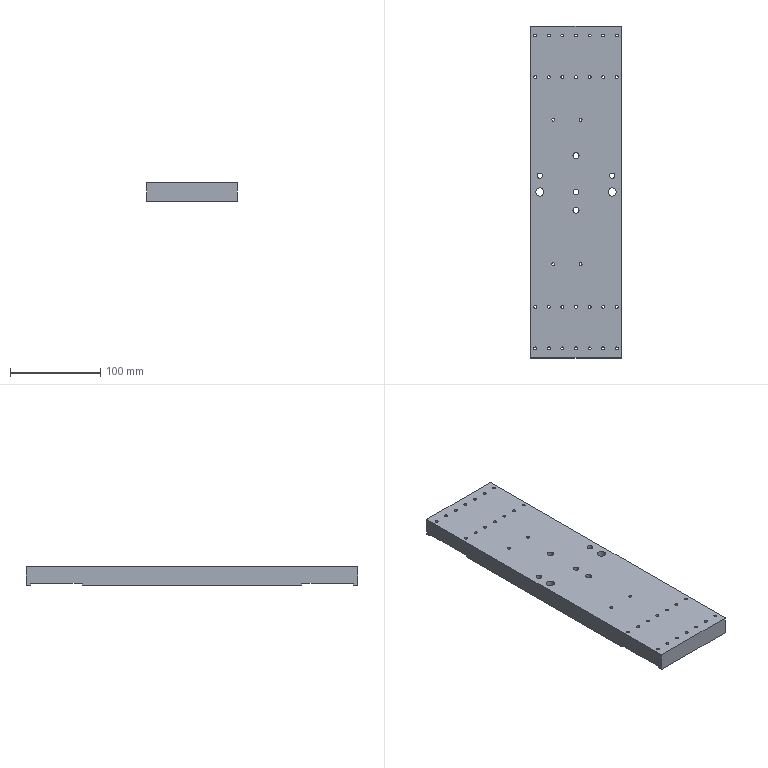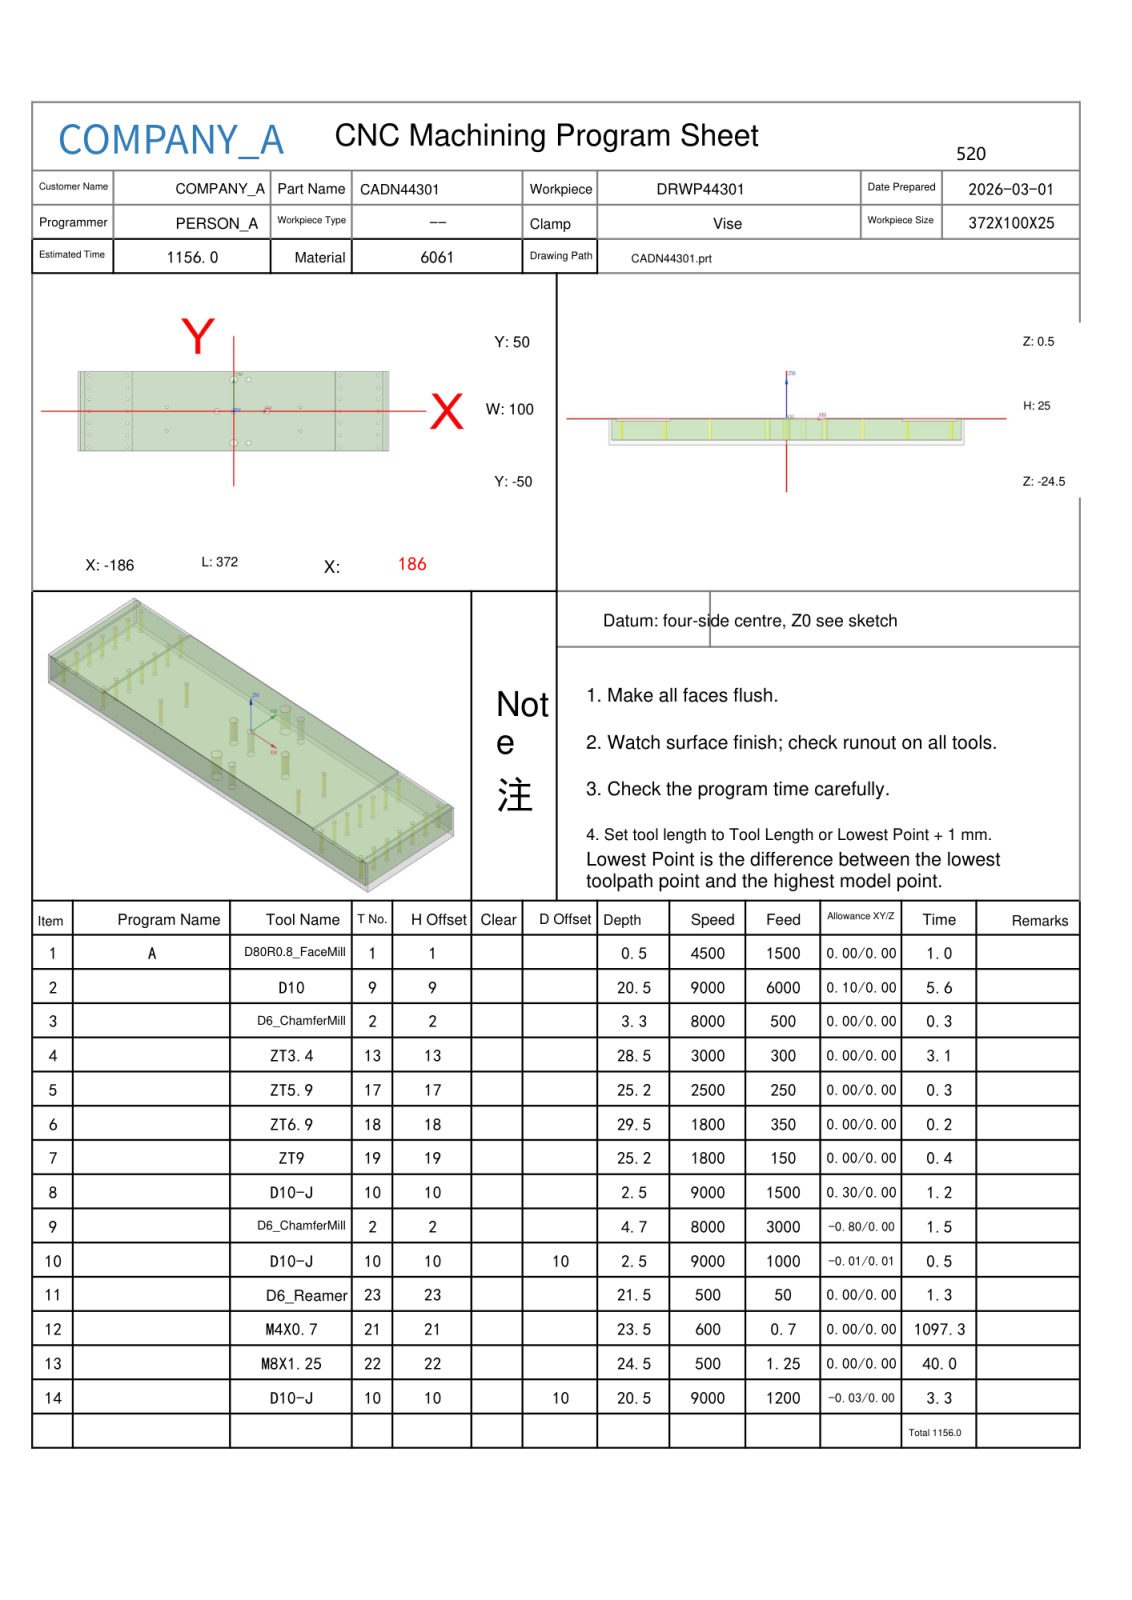NC program | NX | posted by the shop | part box 100 x 367 x 20 mm
Whole program:
%
O0001
(Machine time: 2248.24 MIN)
(===Total Tool:11===)
(T1=D80R0.8 FaceMill D=80.  R=0.8  D-  H01 Z=0.    )
(T9=D10     D=10.  R=0.   D-  H09 Z=-20.  )
(T2=D6_ChamferMill   D=6.   R=0.   D-  H02 Z=-4.2  )
(T13=ZT3.4  D=3.4  DR_a=118 D-  H13 Z=-28.  )
(T17=ZT5.9  D=5.9  DR_a=120 D-  H17 Z=-24.7 )
(T18=ZT6.9  D=6.9  DR_a=120 D-  H18 Z=-29.  )
(T19=ZT9    D=9.   DR_a=118 D-  H19 Z=-24.7 )
(T10=D10-J  D=10.  R=0.   D-  H10 Z=-20.  )
(T23=D6_Reamer   D=6.   DR_a=180 D23 H23 Z=-21.  )
(T21=M4X0.7 D=3.3  DR_a=180 D-  H21 Z=-23.  )
(T22=M8X1.25 D=6.8  DR_a=180 D-  H22 Z=-24.  )
G80 G90 G17 G49 G40
G91 G28 Z0
M01
N1 T01 M06
(D80R0.8 FaceMill  D=80. R=0.8 H=01 ce=0.00 di=0.00)
G00 G90 G54 X-228.5 Y45. M03 S4500
G43 H01 Z50.
M08
Z2.
G01 Z0.0 F1500.
X-223.5
X223.5
Y0.0
X-223.5
Y-45.
X223.5
X228.5
Z2.
G00 Z50.
G91 G28 Z0.0
M05
M09
G91 G28 Z0.0
M01
N2 T09 M06
(D10  D=10. R=0. H=09 ce=0.10 di=0.00)
G00 G90 G54 X0.0 Y55.1 M03 S8000
G43 H09 Z50.
M08
Z.5
G01 X183.5 Z.35 F6000.
G02 X188.6 Y50. Z.344 I0.0 J-5.1
G01 Y-50. Z.262
G02 X183.5 Y-55.1 Z.256 I-5.1 J0.0
G01 X-183.5 Z-.044
G02 X-188.6 Y-50. Z-.051 I0.0 J5.1
G01 Y50. Z-.132
G02 X-183.5 Y55.1 Z-.139 I5.1 J0.0
G01 X183.5 Z-.438
G02 X188.6 Y50. Z-.445 I0.0 J-5.1
G01 Y-50. Z-.526
G02 X183.5 Y-55.1 Z-.533 I-5.1 J0.0
G01 X-183.5 Z-.832
G02 X-188.6 Y-50. Z-.839 I0.0 J5.1
G01 Y50. Z-.921
G02 X-183.5 Y55.1 Z-.927 I5.1 J0.0
G01 X183.5 Z-1.227
G02 X188.6 Y50. Z-1.233 I0.0 J-5.1
G01 Y-50. Z-1.315
G02 X183.5 Y-55.1 Z-1.321 I-5.1 J0.0
G01 X-183.5 Z-1.621
G02 X-188.6 Y-50. Z-1.627 I0.0 J5.1
G01 Y50. Z-1.709
G02 X-183.5 Y55.1 Z-1.716 I5.1 J0.0
G01 X183.5 Z-2.015
G02 X188.6 Y50. Z-2.022 I0.0 J-5.1
G01 Y-50. Z-2.103
G02 X183.5 Y-55.1 Z-2.11 I-5.1 J0.0
G01 X-183.5 Z-2.409
G02 X-188.6 Y-50. Z-2.416 I0.0 J5.1
G01 Y50. Z-2.498
G02 X-183.5 Y55.1 Z-2.504 I5.1 J0.0
G01 X183.5 Z-2.804
G02 X188.6 Y50. Z-2.81 I0.0 J-5.1
G01 Y-50. Z-2.892
G02 X183.5 Y-55.1 Z-2.898 I-5.1 J0.0
G01 X-183.5 Z-3.198
G02 X-188.6 Y-50. Z-3.204 I0.0 J5.1
G01 Y50. Z-3.286
G02 X-183.5 Y55.1 Z-3.293 I5.1 J0.0
G01 X183.5 Z-3.592
G02 X188.6 Y50. Z-3.599 I0.0 J-5.1
G01 Y-50. Z-3.68
G02 X183.5 Y-55.1 Z-3.687 I-5.1 J0.0
G01 X-183.5 Z-3.986
G02 X-188.6 Y-50. Z-3.993 I0.0 J5.1
G01 Y50. Z-4.074
G02 X-183.5 Y55.1 Z-4.081 I5.1 J0.0
G01 X183.5 Z-4.381
G02 X188.6 Y50. Z-4.387 I0.0 J-5.1
G01 Y-50. Z-4.469
G02 X183.5 Y-55.1 Z-4.475 I-5.1 J0.0
G01 X-183.5 Z-4.775
G02 X-188.6 Y-50. Z-4.781 I0.0 J5.1
G01 Y50. Z-4.863
G02 X-183.5 Y55.1 Z-4.869 I5.1 J0.0
G01 X183.5 Z-5.169
G02 X188.6 Y50. Z-5.176 I0.0 J-5.1
G01 Y-50. Z-5.257
G02 X183.5 Y-55.1 Z-5.264 I-5.1 J0.0
G01 X-183.5 Z-5.563
G02 X-188.6 Y-50. Z-5.57 I0.0 J5.1
G01 Y50. Z-5.651
G02 X-183.5 Y55.1 Z-5.658 I5.1 J0.0
G01 X183.5 Z-5.957
G02 X188.6 Y50. Z-5.964 I0.0 J-5.1
G01 Y-50. Z-6.046
G02 X183.5 Y-55.1 Z-6.052 I-5.1 J0.0
G01 X-183.5 Z-6.352
G02 X-188.6 Y-50. Z-6.358 I0.0 J5.1
G01 Y50. Z-6.44
G02 X-183.5 Y55.1 Z-6.446 I5.1 J0.0
G01 X183.5 Z-6.746
G02 X188.6 Y50. Z-6.752 I0.0 J-5.1
G01 Y-50. Z-6.834
G02 X183.5 Y-55.1 Z-6.841 I-5.1 J0.0
G01 X-183.5 Z-7.14
G02 X-188.6 Y-50. Z-7.147 I0.0 J5.1
G01 Y50. Z-7.228
G02 X-183.5 Y55.1 Z-7.235 I5.1 J0.0
G01 X183.5 Z-7.534
G02 X188.6 Y50. Z-7.541 I0.0 J-5.1
G01 Y-50. Z-7.623
G02 X183.5 Y-55.1 Z-7.629 I-5.1 J0.0
G01 X-183.5 Z-7.929
G02 X-188.6 Y-50. Z-7.935 I0.0 J5.1
G01 Y50. Z-8.017
G02 X-183.5 Y55.1 Z-8.023 I5.1 J0.0
G01 X183.5 Z-8.323
G02 X188.6 Y50. Z-8.329 I0.0 J-5.1
G01 Y-50. Z-8.411
G02 X183.5 Y-55.1 Z-8.418 I-5.1 J0.0
G01 X-183.5 Z-8.717
G02 X-188.6 Y-50. Z-8.724 I0.0 J5.1
G01 Y50. Z-8.805
G02 X-183.5 Y55.1 Z-8.812 I5.1 J0.0
G01 X183.5 Z-9.111
G02 X188.6 Y50. Z-9.118 I0.0 J-5.1
G01 Y-50. Z-9.199
G02 X183.5 Y-55.1 Z-9.206 I-5.1 J0.0
G01 X-183.5 Z-9.506
G02 X-188.6 Y-50. Z-9.512 I0.0 J5.1
G01 Y50. Z-9.594
G02 X-183.5 Y55.1 Z-9.6 I5.1 J0.0
G01 X183.5 Z-9.9
G02 X188.6 Y50. Z-9.906 I0.0 J-5.1
G01 Y-50. Z-9.988
G02 X183.5 Y-55.1 Z-9.994 I-5.1 J0.0
G01 X-183.5 Z-10.294
G02 X-188.6 Y-50. Z-10.301 I0.0 J5.1
G01 Y50. Z-10.382
G02 X-183.5 Y55.1 Z-10.389 I5.1 J0.0
G01 X183.5 Z-10.688
G02 X188.6 Y50. Z-10.695 I0.0 J-5.1
G01 Y-50. Z-10.776
G02 X183.5 Y-55.1 Z-10.783 I-5.1 J0.0
G01 X-183.5 Z-11.082
G02 X-188.6 Y-50. Z-11.089 I0.0 J5.1
G01 Y50. Z-11.171
G02 X-183.5 Y55.1 Z-11.177 I5.1 J0.0
G01 X183.5 Z-11.477
G02 X188.6 Y50. Z-11.483 I0.0 J-5.1
G01 Y-50. Z-11.565
G02 X183.5 Y-55.1 Z-11.571 I-5.1 J0.0
G01 X-183.5 Z-11.871
G02 X-188.6 Y-50. Z-11.877 I0.0 J5.1
G01 Y50. Z-11.959
G02 X-183.5 Y55.1 Z-11.966 I5.1 J0.0
G01 X183.5 Z-12.265
G02 X188.6 Y50. Z-12.272 I0.0 J-5.1
G01 Y-50. Z-12.353
G02 X183.5 Y-55.1 Z-12.36 I-5.1 J0.0
G01 X-183.5 Z-12.659
G02 X-188.6 Y-50. Z-12.666 I0.0 J5.1
G01 Y50. Z-12.748
G02 X-183.5 Y55.1 Z-12.754 I5.1 J0.0
G01 X183.5 Z-13.054
G02 X188.6 Y50. Z-13.06 I0.0 J-5.1
G01 Y-50. Z-13.142
G02 X183.5 Y-55.1 Z-13.148 I-5.1 J0.0
G01 X-183.5 Z-13.448
G02 X-188.6 Y-50. Z-13.454 I0.0 J5.1
G01 Y50. Z-13.536
G02 X-183.5 Y55.1 Z-13.543 I5.1 J0.0
G01 X183.5 Z-13.842
G02 X188.6 Y50. Z-13.849 I0.0 J-5.1
G01 Y-50. Z-13.93
G02 X183.5 Y-55.1 Z-13.937 I-5.1 J0.0
G01 X-183.5 Z-14.236
G02 X-188.6 Y-50. Z-14.243 I0.0 J5.1
G01 Y50. Z-14.324
G02 X-183.5 Y55.1 Z-14.331 I5.1 J0.0
G01 X183.5 Z-14.631
G02 X188.6 Y50. Z-14.637 I0.0 J-5.1
G01 Y-50. Z-14.719
G02 X183.5 Y-55.1 Z-14.725 I-5.1 J0.0
G01 X-183.5 Z-15.025
G02 X-188.6 Y-50. Z-15.031 I0.0 J5.1
G01 Y50. Z-15.113
G02 X-183.5 Y55.1 Z-15.119 I5.1 J0.0
G01 X183.5 Z-15.419
G02 X188.6 Y50. Z-15.426 I0.0 J-5.1
G01 Y-50. Z-15.507
G02 X183.5 Y-55.1 Z-15.514 I-5.1 J0.0
G01 X-183.5 Z-15.813
G02 X-188.6 Y-50. Z-15.82 I0.0 J5.1
G01 Y50. Z-15.901
G02 X-183.5 Y55.1 Z-15.908 I5.1 J0.0
G01 X183.5 Z-16.207
G02 X188.6 Y50. Z-16.214 I0.0 J-5.1
G01 Y-50. Z-16.296
G02 X183.5 Y-55.1 Z-16.302 I-5.1 J0.0
G01 X-183.5 Z-16.602
G02 X-188.6 Y-50. Z-16.608 I0.0 J5.1
G01 Y50. Z-16.69
G02 X-183.5 Y55.1 Z-16.696 I5.1 J0.0
G01 X183.5 Z-16.996
G02 X188.6 Y50. Z-17.002 I0.0 J-5.1
G01 Y-50. Z-17.084
G02 X183.5 Y-55.1 Z-17.091 I-5.1 J0.0
G01 X-183.5 Z-17.39
G02 X-188.6 Y-50. Z-17.397 I0.0 J5.1
G01 Y50. Z-17.478
G02 X-183.5 Y55.1 Z-17.485 I5.1 J0.0
G01 X183.5 Z-17.784
G02 X188.6 Y50. Z-17.791 I0.0 J-5.1
G01 Y-50. Z-17.873
G02 X183.5 Y-55.1 Z-17.879 I-5.1 J0.0
G01 X-183.5 Z-18.179
G02 X-188.6 Y-50. Z-18.185 I0.0 J5.1
G01 Y50. Z-18.267
G02 X-183.5 Y55.1 Z-18.273 I5.1 J0.0
G01 X183.5 Z-18.573
G02 X188.6 Y50. Z-18.579 I0.0 J-5.1
G01 Y-50. Z-18.661
G02 X183.5 Y-55.1 Z-18.668 I-5.1 J0.0
G01 X-183.5 Z-18.967
G02 X-188.6 Y-50. Z-18.974 I0.0 J5.1
G01 Y50. Z-19.055
G02 X-183.5 Y55.1 Z-19.062 I5.1 J0.0
G01 X183.5 Z-19.361
G02 X188.6 Y50. Z-19.368 I0.0 J-5.1
G01 Y-50. Z-19.449
G02 X183.5 Y-55.1 Z-19.456 I-5.1 J0.0
G01 X-183.5 Z-19.756
G02 X-188.6 Y-50. Z-19.762 I0.0 J5.1
G01 Y50. Z-19.844
G02 X-183.5 Y55.1 Z-19.85 I5.1 J0.0
G01 X0.0 Z-20.
X183.5
G02 X188.6 Y50. I0.0 J-5.1
G01 Y-50.
G02 X183.5 Y-55.1 I-5.1 J0.0
G01 X-183.5
G02 X-188.6 Y-50. I0.0 J5.1
G01 Y50.
G02 X-183.5 Y55.1 I5.1 J0.0
G01 X0.0
X.5
Z-19.
G00 Z50.
G00 G90 X-150. Y58. M03 S9000
Z50.
Z.025
G01 Z-.475 F6000.
Y51.
X-126.6
Y-51.
X-173.4
Y51.
X-150.
Y44.
X-133.6
Y-44.
X-166.4
Y44.
X-150.
Y37.
X-140.6
Y-37.
X-159.4
Y37.
X-150.
Y30.
X-147.6
Y-30.
X-152.4
Y30.
X-150.
X-149.5
Z.025
G00 Z.5
X-150. Y58.
Z-.45
G01 Z-.95
Y51.
X-126.6
Y-51.
X-173.4
Y51.
X-150.
Y44.
X-133.6
Y-44.
X-166.4
Y44.
X-150.
Y37.
X-140.6
Y-37.
X-159.4
Y37.
X-150.
Y30.
X-147.6
Y-30.
X-152.4
Y30.
X-150.
X-149.5
Z-.45
G00 Z.025
X-150. Y58.
Z-.925
G01 Z-1.425
Y51.
X-126.6
Y-51.
X-173.4
Y51.
X-150.
Y44.
X-133.6
Y-44.
X-166.4
Y44.
X-150.
Y37.
X-140.6
Y-37.
X-159.4
Y37.
X-150.
Y30.
X-147.6
Y-30.
X-152.4
Y30.
X-150.
X-149.5
Z-.925
G00 Z-.45
X-150. Y58.
Z-1.4
G01 Z-1.9
Y51.
X-126.6
Y-51.
X-173.4
Y51.
X-150.
Y44.
X-133.6
Y-44.
X-166.4
Y44.
X-150.
Y37.
X-140.6
Y-37.
X-159.4
Y37.
X-150.
Y30.
X-147.6
Y-30.
X-152.4
Y30.
X-150.
X-149.5
Z-1.4
G00 Z50.
X150. Y58.
Z.025
G01 Z-.475
Y51.
X173.4
Y-51.
X126.6
Y51.
X150.
Y44.
X166.4
Y-44.
X133.6
Y44.
X150.
Y37.
X159.4
Y-37.
X140.6
Y37.
X150.
Y30.
X152.4
Y-30.
X147.6
Y30.
X150.
X150.5
Z.025
G00 Z.5
X150. Y58.
Z-.45
G01 Z-.95
Y51.
X173.4
Y-51.
X126.6
Y51.
X150.
Y44.
X166.4
Y-44.
X133.6
Y44.
X150.
Y37.
X159.4
Y-37.
X140.6
Y37.
X150.
Y30.
X152.4
Y-30.
X147.6
Y30.
X150.
X150.5
Z-.45
G00 Z.025
X150. Y58.
Z-.925
G01 Z-1.425
Y51.
X173.4
Y-51.
X126.6
Y51.
X150.
Y44.
X166.4
Y-44.
X133.6
Y44.
X150.
Y37.
X159.4
Y-37.
X140.6
Y37.
X150.
Y30.
X152.4
Y-30.
X147.6
Y30.
X150.
X150.5
Z-.925
G00 Z-.45
X150. Y58.
Z-1.4
G01 Z-1.9
Y51.
X173.4
Y-51.
X126.6
Y51.
X150.
Y44.
X166.4
Y-44.
X133.6
Y44.
X150.
Y37.
X159.4
Y-37.
X140.6
Y37.
X150.
Y30.
X152.4
Y-30.
X147.6
Y30.
X150.
X150.5
Z-1.4
G00 Z50.
G91 G28 Z0.0
M05
M09
G91 G28 Z0.0
M01
N3 T02 M06
(D6_ChamferMill  D=6. R=0. H=02 ce=0.00 di=0.10)
G00 G90 G54 X173. Y-45. M03 S8000
G43 H02 Z50.
M08
G98 G81 X173. Y-45. Z-2.8 R-1. F500.
Y-30.
Y-15.
Y0.0
Y15.
Y30.
Y45.
X127.
Y30.
Y15.
Y0.0
Y-15.
Y-30.
Y-45.
X80. Y-25. Z-.8 R1.
Y5.
X40. Y0.0
X18. Y40.
X0.0
Y0.0
X18. Y-40.
X0.0
X-20. Y0.0
X-80. Y-25.
Y5.
X-127. Y45. Z-2.8 R-1.
Y30.
Y15.
Y0.0
Y-15.
Y-30.
Y-45.
X-173.
Y-30.
Y-15.
Y0.0
Y15.
Y30.
Y45.
G80
G00 Z50.
G91 G28 Z0.0
M05
M09
G91 G28 Z0.0
M01
N4 T13 M06
(ZT3.4 D=3.4 DR_a=118 H=13)
G00 G90 G54 X-173. Y-45. M03 S3000
G43 H13 Z50.
M08
G98 G83 X-173. Y-45. Z-28. R-1. F300. Q2.
Y-30.
Y-15.
Y0.0
Y15.
Y30.
Y45.
X-127.
Y30.
Y15.
Y0.0
Y-15.
Y-30.
Y-45.
X-80. Y-25. Z-26. R1.
Y5.
X80.
Y-25.
X127. Y-45. Z-28. R-1.
Y-30.
Y-15.
Y0.0
Y15.
Y30.
Y45.
X173.
Y30.
Y15.
Y0.0
Y-15.
Y-30.
Y-45.
G80
G00 Z50.
G91 G28 Z0.0
M05
M09
G91 G28 Z0.0
M01
N5 T17 M06
(ZT5.9 D=5.9 DR_a=120 H=17)
G00 G90 G54 X18. Y40. M03 S2500
G43 H17 Z50.
M08
G98 G83 X18. Y40. Z-24.703 R1. F250. Q2.
X0.0 Y0.0
X18. Y-40.
G80
G00 Z50.
G91 G28 Z0.0
M05
M09
G91 G28 Z0.0
M01
N6 T18 M06
(ZT6.9 D=6.9 DR_a=120 H=18)
G00 G90 G54 X-20. Y0.0 M03 S1800
G43 H18 Z50.
M08
G98 G83 X-20. Y0.0 Z-29. R1. F350. Q3.
X40.
G80
G00 Z50.
G91 G28 Z0.0
M05
M09
G91 G28 Z0.0
M01
N7 T19 M06
(ZT9 D=9. DR_a=118 H=19)
G00 G90 G54 X0.0 Y40. M03 S1800
G43 H19 Z50.
M08
G98 G83 X0.0 Y40. Z-24.704 R1. F150. Q3.
Y-40.
G80
G00 Z50.
G91 G28 Z0.0
M05
M09
G91 G28 Z0.0
M01
N8 T10 M06
(D10-J  D=10. R=0. H=10 ce=0.30 di=0.00)
G00 G90 G54 X-150. Y58. M03 S9000
G43 H10 Z50.
M08
Z-1.5
G01 Z-2. F1500.
Y51.
X-126.8
Y-51.
X-173.2
Y51.
X-150.
Y44.
X-133.8
Y-44.
X-166.2
Y44.
X-150.
Y37.
X-140.8
Y-37.
X-159.2
Y37.
X-150.
Y30.
X-147.8
Y-30.
X-152.2
Y30.
X-150.
X-149.5
Y36.
Z-1.5
G00 Z50.
X150. Y58.
Z-1.5
G01 Z-2.
Y51.
X173.2
Y-51.
X126.8
Y51.
X150.
Y44.
X166.2
Y-44.
X133.8
Y44.
X150.
Y37.
X159.2
Y-37.
X140.8
Y37.
X150.
Y30.
X152.2
Y-30.
X147.8
Y30.
X150.
X150.5
Y36.
Z-1.5
G00 Z50.
G91 G28 Z0.0
M05
M09
G91 G28 Z0.0
M01
N9 T02 M06
(D6_ChamferMill  D=6. R=0. H=02 ce=0.00 di=0.00)
G00 G90 G54 X176.372 Y-.25 M03 S8000
G43 H02 Z50.
M08
Z2.099
G01 Z-1.5 F3000.
G03 X176.672 Y-.33 I.3 J.52
X177.192 Y-.03 I0.0 J.6
G01 X177.2 Y0.0
Y50.
G02 X178.5 Y51.3 I1.3 J0.0
G01 X183.5
G02 X184.8 Y50. I0.0 J-1.3
G01 Y-50.
G02 X183.5 Y-51.3 I-1.3 J0.0
G01 X178.5
G02 X177.2 Y-50. I0.0 J1.3
G01 Y0.0
X177.192 Y.03
G03 X176.672 Y.33 I-.52 J-.3
X176.372 Y.25 I0.0 J-.6
G01 Z2.099
G00 Z50.
X.25 Y-52.128
Z2.099
G01 Z-1.5
G03 X.33 Y-51.828 I-.52 J.3
X.03 Y-51.308 I-.6 J0.0
G01 X0.0 Y-51.3
X-121.5
G02 X-122.8 Y-50. I0.0 J1.3
G01 Y50.
G02 X-121.5 Y51.3 I1.3 J0.0
G01 X121.5
G02 X122.8 Y50. I0.0 J-1.3
G01 Y-50.
G02 X121.5 Y-51.3 I-1.3 J0.0
G01 X0.0
X-.03 Y-51.308
G03 X-.33 Y-51.828 I.3 J-.52
X-.25 Y-52.128 I.6 J0.0
G01 Z2.099
G00 Z50.
X-176.372 Y.25
Z2.099
G01 Z-1.5
G03 X-176.672 Y.33 I-.3 J-.52
X-177.192 Y.03 I0.0 J-.6
G01 X-177.2 Y0.0
Y-50.
G02 X-178.5 Y-51.3 I-1.3 J0.0
G01 X-183.5
G02 X-184.8 Y-50. I0.0 J1.3
G01 Y50.
G02 X-183.5 Y51.3 I1.3 J0.0
G01 X-178.5
G02 X-177.2 Y50. I0.0 J-1.3
G01 Y0.0
X-177.192 Y-.03
G03 X-176.672 Y-.33 I.52 J.3
X-176.372 Y-.25 I0.0 J.6
G01 Z2.099
G00 Z50.
X-175.465 Y52.128
Z1.755
G01 Z-3.499
G03 X-175.546 Y51.828 I.52 J-.3
X-175.246 Y51.308 I.6 J0.0
G01 X-175.216 Y51.3
X-124.784
X-124.754 Y51.308
G03 X-124.454 Y51.828 I-.3 J.52
X-124.535 Y52.128 I-.6 J0.0
G01 Z1.755
G00 Z50.
Y-52.128
Z1.755
G01 Z-3.499
G03 X-124.454 Y-51.828 I-.52 J.3
X-124.754 Y-51.308 I-.6 J0.0
G01 X-124.784 Y-51.3
X-175.216
X-175.246 Y-51.308
G03 X-175.546 Y-51.828 I.3 J-.52
X-175.465 Y-52.128 I.6 J0.0
G01 Z1.755
G00 Z50.
X175.465
Z1.755
G01 Z-3.499
G03 X175.546 Y-51.828 I-.52 J.3
X175.246 Y-51.308 I-.6 J0.0
G01 X175.216 Y-51.3
X124.784
X124.754 Y-51.308
G03 X124.454 Y-51.828 I.3 J-.52
X124.535 Y-52.128 I.6 J0.0
G01 Z1.755
G00 Z50.
Y52.128
Z1.755
G01 Z-3.499
G03 X124.454 Y51.828 I.52 J-.3
X124.754 Y51.308 I.6 J0.0
G01 X124.784 Y51.3
X175.216
X175.246 Y51.308
G03 X175.546 Y51.828 I-.3 J.52
X175.465 Y52.128 I-.6 J0.0
G01 Z1.755
G00 Z50.
G00 G90 X-173. Y-45. M03 S8000
Z50.
G98 G81 X-173. Y-45. Z-4.2 R1. F500.
Y-30.
Y-15.
Y0.0
Y15.
Y30.
Y45.
X-127.
Y30.
Y15.
Y0.0
Y-15.
Y-30.
Y-45.
X-80. Y-25. Z-2.2 R3.
Y5.
X80.
Y-25.
X127. Y-45. Z-4.2 R1.
Y-30.
Y-15.
Y0.0
Y15.
Y30.
Y45.
X173.
Y30.
Y15.
Y0.0
Y-15.
Y-30.
Y-45.
G80
G00 Z50.
G00 G90 X19.147 Y-39.388 M03 S8000
Z50.
Z-.5
G01 Z-1. F500.
X19.5 Y-39.2
G03 X18. Y-37.7 I-1.5 J0.0
X15.7 Y-40. I0.0 J-2.3
X18. Y-42.3 I2.3 J0.0
X20.3 Y-40. I0.0 J2.3
X18. Y-37.7 I-2.3 J0.0
X16.5 Y-39.2 I0.0 J-1.5
G01 X16.853 Y-39.388
Z-.5
G00 Z50.
X1.147 Y.612
Z-.5
G01 Z-1.
X1.5 Y.8
G03 X0.0 Y2.3 I-1.5 J0.0
X-2.3 Y0.0 I0.0 J-2.3
X0.0 Y-2.3 I2.3 J0.0
X2.3 Y0.0 I0.0 J2.3
X0.0 Y2.3 I-2.3 J0.0
X-1.5 Y.8 I0.0 J-1.5
G01 X-1.147 Y.612
Z-.5
G00 Z50.
X19.147 Y40.612
Z-.5
G01 Z-1.
X19.5 Y40.8
G03 X18. Y42.3 I-1.5 J0.0
X15.7 Y40. I0.0 J-2.3
X18. Y37.7 I2.3 J0.0
X20.3 Y40. I0.0 J2.3
X18. Y42.3 I-2.3 J0.0
X16.5 Y40.8 I0.0 J-1.5
G01 X16.853 Y40.612
Z-.5
G00 Z50.
G00 G90 X-18.5 Y1.166 M03 S8000
Z50.
Z-.8
G01 Z-1.3 F600.
Y1.4
G03 X-20. Y2.9 I-1.5 J0.0
X-22.9 Y0.0 I0.0 J-2.9
X-20. Y-2.9 I2.9 J0.0
X-17.1 Y0.0 I0.0 J2.9
X-20. Y2.9 I-2.9 J0.0
X-21.5 Y1.4 I0.0 J-1.5
G01 Y1.166
Z-.8
G00 Z50.
X41.5
Z-.8
G01 Z-1.3
Y1.4
G03 X40. Y2.9 I-1.5 J0.0
X37.1 Y0.0 I0.0 J-2.9
X40. Y-2.9 I2.9 J0.0
X42.9 Y0.0 I0.0 J2.9
X40. Y2.9 I-2.9 J0.0
X38.5 Y1.4 I0.0 J-1.5
G01 Y1.166
Z-.8
G00 Z50.
G00 G90 X-2.705 Y39.279 M03 S8000
Z50.
Z-.5
G01 Z-1. F800.
X-3. Y39.2
G03 X0.0 Y36.2 I3. J0.0
X3.8 Y40. I0.0 J3.8
X0.0 Y43.8 I-3.8 J0.0
X-3.8 Y40. I0.0 J-3.8
X0.0 Y36.2 I3.8 J0.0
X3. Y39.2 I0.0 J3.
G01 X2.705 Y39.279
Z-.5
G00 Z50.
X-2.705 Y-40.721
Z-.5
G01 Z-1.
X-3. Y-40.8
G03 X0.0 Y-43.8 I3. J0.0
X3.8 Y-40. I0.0 J3.8
X0.0 Y-36.2 I-3.8 J0.0
X-3.8 Y-40. I0.0 J-3.8
X0.0 Y-43.8 I3.8 J0.0
X3. Y-40.8 I0.0 J3.
G01 X2.705 Y-40.721
Z-.5
G00 Z50.
G91 G28 Z0.0
M05
M09
G91 G28 Z0.0
M01
N10 T10 M06
(D10-J  D=10. R=0. H=10 ce=-0.01 di=0.01)
G00 G90 G54 X127.59 Y55.5 M03 S9000
G43 H10 Z50.
M08
Z-1.495
G01 Z-1.995 F1000.
G41 D10
X127.49
G03 X126.49 Y54.5 I0.0 J-1.
G01 Y-54.5
G03 X127.49 Y-55.5 I1. J0.0
G01 G40 X127.59
Z-1.495
G00 Z50.
X172.41
Z-1.495
G01 Z-1.995
G41 D10
X172.51
G03 X173.51 Y-54.5 I0.0 J1.
G01 Y54.5
G03 X172.51 Y55.5 I-1. J0.0
G01 G40 X172.41
Z-1.495
G00 Z50.
X-127.59 Y-55.5
Z-1.495
G01 Z-1.995
G41 D10
X-127.49
G03 X-126.49 Y-54.5 I0.0 J1.
G01 Y54.5
G03 X-127.49 Y55.5 I-1. J0.0
G01 G40 X-127.59
Z-1.495
G00 Z50.
X-172.41
Z-1.495
G01 Z-1.995
G41 D10
X-172.51
G03 X-173.51 Y54.5 I0.0 J-1.
G01 Y-54.5
G03 X-172.51 Y-55.5 I1. J0.0
G01 G40 X-172.41
Z-1.495
G00 Z50.
G91 G28 Z0.0
M05
M09
G91 G28 Z0.0
M01
N11 T23 M06
(D6_Reamer D=6. DR_a=180 H=23)
G00 G90 G54 X18. Y40. M03 S500
G43 H23 Z50.
M08
G98 G81 X18. Y40. Z-21. R1. F50.
X0.0 Y0.0
X18. Y-40.
G80
G00 Z50.
G91 G28 Z0.0
M05
M09
G91 G28 Z0.0
M01
N12 T21 M06
(M4X0.7 D=3.3 DR_a=180 H=21)
G00 G90 G54 X-173. Y-45. M03 S600
G43 H21 Z50.
M08
G95
G98 G84 X-173. Y-45. Z-23. R1. F.7 Q4.
Y-30.
Y-15.
Y0.0
Y15.
Y30.
Y45.
X-127.
Y30.
Y15.
Y0.0
Y-15.
Y-30.
Y-45.
X-80. Y-25.
Y5.
X80.
Y-25.
X127. Y-45.
Y-30.
Y-15.
Y0.0
Y15.
Y30.
Y45.
X173.
Y30.
Y15.
Y0.0
Y-15.
Y-30.
Y-45.
G80
G94
G00 Z50.
G91 G28 Z0.0
M05
M09
G91 G28 Z0.0
M01
N13 T22 M06
(M8X1.25 D=6.8 DR_a=180 H=22)
G00 G90 G54 X-20. Y0.0 M03 S500
G43 H22 Z50.
M08
G95
G98 G84 X-20. Y0.0 Z-24. R1. F1.25 Q4.
X40.
G80
G94
G00 Z50.
G91 G28 Z0.0
M05
M09
G91 G28 Z0.0
M01
N14 T10 M06
(D10-J  D=10. R=0. H=10 ce=0.00 di=0.00)
G00 G90 G54 X-184.513 Y56.116 M03 S9000
G43 H10 Z50.
M08
Z-9.5
G01 Z-10. F1200.
G41 D10
X-184.497 Y55.917
G03 X-183.5 Y55. I.997 J.083
G01 X183.5
G02 X188.5 Y50. I0.0 J-5.
G01 Y-50.
G02 X183.5 Y-55. I-5. J0.0
G01 X-183.5
G02 X-188.5 Y-50. I0.0 J5.
G01 Y50.
G02 X-183.5 Y55. I5. J0.0
G01 X-183.
G03 X-182. Y56. I0.0 J1.
G01 G40 Y56.2
Z-9.5
G00 Z50.
X-184.513 Y56.116
Z-19.5
G01 Z-20.
G41 D10
X-184.497 Y55.917
G03 X-183.5 Y55. I.997 J.083
G01 X183.5
G02 X188.5 Y50. I0.0 J-5.
G01 Y-50.
G02 X183.5 Y-55. I-5. J0.0
G01 X-183.5
G02 X-188.5 Y-50. I0.0 J5.
G01 Y50.
G02 X-183.5 Y55. I5. J0.0
G01 X-183.
G03 X-182. Y56. I0.0 J1.
G01 G40 Y56.2
Z-19.5
G00 Z50.
G00 G90 X-190.011 Y56.399 M03 S8000
Z10.5
Z-8.5
G01 Z-10. F1000.
G41 D10
X-189.975 Y56.202
G03 X-188.5 Y54.975 I1.475 J.273
G01 X188.5
G03 X189.975 Y56.202 I0.0 J1.5
G01 G40 X190.011 Y56.399
Z-8.5
G00 Z3.
X-190.011
Z-18.5
G01 Z-20.
G41 D10
X-189.975 Y56.202
G03 X-188.5 Y54.975 I1.475 J.273
G01 X188.5
G03 X189.975 Y56.202 I0.0 J1.5
G01 G40 X190.011 Y56.399
Z-18.5
G00 Z10.5
Y-56.399
Z-8.5
G01 Z-10.
G41 D10
X189.975 Y-56.202
G03 X188.5 Y-54.975 I-1.475 J-.273
G01 X-188.5
G03 X-189.975 Y-56.202 I0.0 J-1.5
G01 G40 X-190.011 Y-56.399
Z-8.5
G00 Z3.
X190.011
Z-18.5
G01 Z-20.
G41 D10
X189.975 Y-56.202
G03 X188.5 Y-54.975 I-1.475 J-.273
G01 X-188.5
G03 X-189.975 Y-56.202 I0.0 J-1.5
G01 G40 X-190.011 Y-56.399
Z-18.5
G00 Z10.5
M05
M09
G91 G28 Z0.0
G91 G28 Y0.0
M30
%